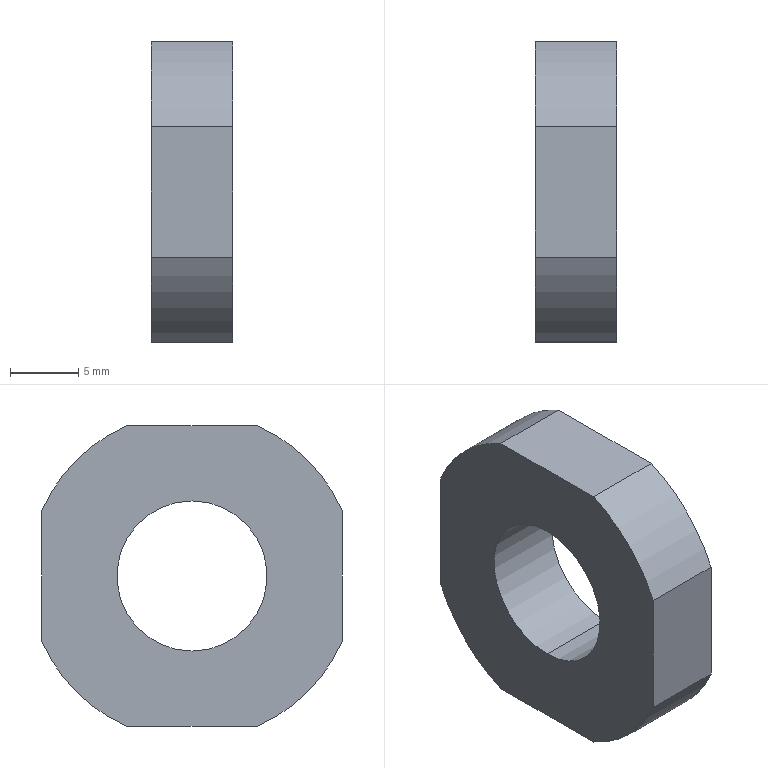Part | STEP file | PN_0031 locking nut | 1 solid | 12 faces | box 6 x 22 x 22 mm | volume 1989 mm3 | cylinder 6 | plane 6 | commonest cylinder face diameters 24 x4 11 x2
STEP:
#1=CARTESIAN_POINT('',(0.,0.,0.));
#2=DIRECTION('',(0.,0.,1.));
#3=DIRECTION('',(1.,0.,0.));
#4=AXIS2_PLACEMENT_3D('',#1,#2,#3);
#5=CARTESIAN_POINT('',(0.,0.,5.5));
#6=VERTEX_POINT('',#5);
#7=CARTESIAN_POINT('',(-6.,0.,5.5));
#8=VERTEX_POINT('',#7);
#9=CARTESIAN_POINT('',(0.,0.,5.5));
#10=DIRECTION('',(-1.,0.,0.));
#11=VECTOR('',#10,1.);
#12=LINE('',#9,#11);
#13=CARTESIAN_POINT('',(0.,0.,0.));
#14=DIRECTION('',(-1.,0.,0.));
#15=DIRECTION('',(0.,0.,1.));
#16=AXIS2_PLACEMENT_3D('',#13,#14,#15);
#17=CYLINDRICAL_SURFACE('',#16,5.5);
#18=CARTESIAN_POINT('',(6.283,0.));
#19=DIRECTION('',(0.,1.));
#20=VECTOR('',#19,1.);
#21=LINE('',#18,#20);
#22=(GEOMETRIC_REPRESENTATION_CONTEXT(2)PARAMETRIC_REPRESENTATION_CONTEXT()REPRESENTATION_CONTEXT('',''));
#23=DEFINITIONAL_REPRESENTATION('',(#21),#22);
#24=PCURVE('',#17,#23);
#25=CARTESIAN_POINT('',(0.,0.,0.));
#26=DIRECTION('',(-1.,0.,0.));
#27=DIRECTION('',(0.,0.,1.));
#28=AXIS2_PLACEMENT_3D('',#25,#26,#27);
#29=CYLINDRICAL_SURFACE('',#28,5.5);
#30=CARTESIAN_POINT('',(0.,0.));
#31=DIRECTION('',(0.,1.));
#32=VECTOR('',#31,1.);
#33=LINE('',#30,#32);
#34=(GEOMETRIC_REPRESENTATION_CONTEXT(2)PARAMETRIC_REPRESENTATION_CONTEXT()REPRESENTATION_CONTEXT('',''));
#35=DEFINITIONAL_REPRESENTATION('',(#33),#34);
#36=PCURVE('',#29,#35);
#37=SURFACE_CURVE('',#12,(#24,#36),.PCURVE_S1.);
#38=EDGE_CURVE('',#6,#8,#37,.T.);
#39=ORIENTED_EDGE('',*,*,#38,.T.);
#40=CARTESIAN_POINT('',(-6.,0.,-5.5));
#41=VERTEX_POINT('',#40);
#42=CARTESIAN_POINT('',(-6.,0.,0.));
#43=DIRECTION('',(1.,0.,0.));
#44=DIRECTION('',(0.,0.,-1.));
#45=AXIS2_PLACEMENT_3D('',#42,#43,#44);
#46=CIRCLE('',#45,5.5);
#47=CARTESIAN_POINT('',(9.425,6.));
#48=DIRECTION('',(-1.,0.));
#49=VECTOR('',#48,1.);
#50=LINE('',#47,#49);
#51=(GEOMETRIC_REPRESENTATION_CONTEXT(2)PARAMETRIC_REPRESENTATION_CONTEXT()REPRESENTATION_CONTEXT('',''));
#52=DEFINITIONAL_REPRESENTATION('',(#50),#51);
#53=PCURVE('',#17,#52);
#54=CARTESIAN_POINT('',(-6.,12.,0.));
#55=DIRECTION('',(-1.,0.,0.));
#56=DIRECTION('',(0.,0.,1.));
#57=AXIS2_PLACEMENT_3D('',#54,#55,#56);
#58=PLANE('',#57);
#59=CARTESIAN_POINT('',(-5.5,-12.));
#60=CARTESIAN_POINT('',(-5.5,-2.474));
#61=CARTESIAN_POINT('',(2.75,-7.237));
#62=CARTESIAN_POINT('',(11.,-12.));
#63=CARTESIAN_POINT('',(2.75,-16.763));
#64=CARTESIAN_POINT('',(-5.5,-21.526));
#65=CARTESIAN_POINT('',(-5.5,-12.));
#66=(BOUNDED_CURVE()B_SPLINE_CURVE(2,(#59,#60,#61,#62,#63,#64,#65),.UNSPECIFIED.,.T.,.F.)B_SPLINE_CURVE_WITH_KNOTS((1,2,2,2,2,1),(-2.094,0.,2.094,4.189,6.283,8.378),.UNSPECIFIED.)CURVE()GEOMETRIC_REPRESENTATION_ITEM()RATIONAL_B_SPLINE_CURVE((1.,0.5,1.,0.5,1.,0.5,1.))REPRESENTATION_ITEM(''));
#67=(GEOMETRIC_REPRESENTATION_CONTEXT(2)PARAMETRIC_REPRESENTATION_CONTEXT()REPRESENTATION_CONTEXT('',''));
#68=DEFINITIONAL_REPRESENTATION('',(#66),#67);
#69=PCURVE('',#58,#68);
#70=SURFACE_CURVE('',#46,(#53,#69),.PCURVE_S1.);
#71=EDGE_CURVE('',#8,#41,#70,.T.);
#72=ORIENTED_EDGE('',*,*,#71,.T.);
#73=CARTESIAN_POINT('',(0.,0.,-5.5));
#74=VERTEX_POINT('',#73);
#75=CARTESIAN_POINT('',(0.,0.,-5.5));
#76=DIRECTION('',(-1.,0.,0.));
#77=VECTOR('',#76,1.);
#78=LINE('',#75,#77);
#79=CARTESIAN_POINT('',(3.142,0.));
#80=DIRECTION('',(0.,1.));
#81=VECTOR('',#80,1.);
#82=LINE('',#79,#81);
#83=(GEOMETRIC_REPRESENTATION_CONTEXT(2)PARAMETRIC_REPRESENTATION_CONTEXT()REPRESENTATION_CONTEXT('',''));
#84=DEFINITIONAL_REPRESENTATION('',(#82),#83);
#85=PCURVE('',#17,#84);
#86=CARTESIAN_POINT('',(3.142,0.));
#87=DIRECTION('',(0.,1.));
#88=VECTOR('',#87,1.);
#89=LINE('',#86,#88);
#90=(GEOMETRIC_REPRESENTATION_CONTEXT(2)PARAMETRIC_REPRESENTATION_CONTEXT()REPRESENTATION_CONTEXT('',''));
#91=DEFINITIONAL_REPRESENTATION('',(#89),#90);
#92=PCURVE('',#29,#91);
#93=SURFACE_CURVE('',#78,(#85,#92),.PCURVE_S1.);
#94=EDGE_CURVE('',#74,#41,#93,.T.);
#95=ORIENTED_EDGE('',*,*,#94,.F.);
#96=CARTESIAN_POINT('',(0.,0.,0.));
#97=DIRECTION('',(1.,0.,0.));
#98=DIRECTION('',(0.,0.,-1.));
#99=AXIS2_PLACEMENT_3D('',#96,#97,#98);
#100=CIRCLE('',#99,5.5);
#101=CARTESIAN_POINT('',(9.425,0.));
#102=DIRECTION('',(-1.,0.));
#103=VECTOR('',#102,1.);
#104=LINE('',#101,#103);
#105=(GEOMETRIC_REPRESENTATION_CONTEXT(2)PARAMETRIC_REPRESENTATION_CONTEXT()REPRESENTATION_CONTEXT('',''));
#106=DEFINITIONAL_REPRESENTATION('',(#104),#105);
#107=PCURVE('',#17,#106);
#108=CARTESIAN_POINT('',(0.,0.,0.));
#109=DIRECTION('',(1.,0.,0.));
#110=DIRECTION('',(0.,0.,-1.));
#111=AXIS2_PLACEMENT_3D('',#108,#109,#110);
#112=PLANE('',#111);
#113=CARTESIAN_POINT('',(0.,0.));
#114=DIRECTION('',(1.,0.));
#115=AXIS2_PLACEMENT_2D('',#113,#114);
#116=CIRCLE('',#115,5.5);
#117=(GEOMETRIC_REPRESENTATION_CONTEXT(2)PARAMETRIC_REPRESENTATION_CONTEXT()REPRESENTATION_CONTEXT('',''));
#118=DEFINITIONAL_REPRESENTATION('',(#116),#117);
#119=PCURVE('',#112,#118);
#120=SURFACE_CURVE('',#100,(#107,#119),.PCURVE_S1.);
#121=EDGE_CURVE('',#6,#74,#120,.T.);
#122=ORIENTED_EDGE('',*,*,#121,.F.);
#123=EDGE_LOOP('',(#39,#72,#95,#122));
#124=FACE_BOUND('',#123,.F.);
#125=ADVANCED_FACE('',(#124),#17,.F.);
#126=CARTESIAN_POINT('',(0.,4.796,11.));
#127=VERTEX_POINT('',#126);
#128=CARTESIAN_POINT('',(-6.,4.796,11.));
#129=VERTEX_POINT('',#128);
#130=CARTESIAN_POINT('',(0.,4.796,11.));
#131=DIRECTION('',(-1.,0.,0.));
#132=VECTOR('',#131,1.);
#133=LINE('',#130,#132);
#134=CARTESIAN_POINT('',(0.,0.,0.));
#135=DIRECTION('',(1.,0.,0.));
#136=DIRECTION('',(0.,0.,-1.));
#137=AXIS2_PLACEMENT_3D('',#134,#135,#136);
#138=CYLINDRICAL_SURFACE('',#137,12.);
#139=CARTESIAN_POINT('',(2.73,0.));
#140=DIRECTION('',(0.,-1.));
#141=VECTOR('',#140,1.);
#142=LINE('',#139,#141);
#143=(GEOMETRIC_REPRESENTATION_CONTEXT(2)PARAMETRIC_REPRESENTATION_CONTEXT()REPRESENTATION_CONTEXT('',''));
#144=DEFINITIONAL_REPRESENTATION('',(#142),#143);
#145=PCURVE('',#138,#144);
#146=CARTESIAN_POINT('',(0.,17.205,11.));
#147=DIRECTION('',(0.,0.,-1.));
#148=DIRECTION('',(0.,1.,0.));
#149=AXIS2_PLACEMENT_3D('',#146,#147,#148);
#150=PLANE('',#149);
#151=CARTESIAN_POINT('',(-12.409,0.));
#152=DIRECTION('',(0.,-1.));
#153=VECTOR('',#152,1.);
#154=LINE('',#151,#153);
#155=(GEOMETRIC_REPRESENTATION_CONTEXT(2)PARAMETRIC_REPRESENTATION_CONTEXT()REPRESENTATION_CONTEXT('',''));
#156=DEFINITIONAL_REPRESENTATION('',(#154),#155);
#157=PCURVE('',#150,#156);
#158=SURFACE_CURVE('',#133,(#145,#157),.PCURVE_S1.);
#159=EDGE_CURVE('',#127,#129,#158,.T.);
#160=ORIENTED_EDGE('',*,*,#159,.F.);
#161=CARTESIAN_POINT('',(0.,11.,4.796));
#162=VERTEX_POINT('',#161);
#163=CARTESIAN_POINT('',(0.,0.,0.));
#164=DIRECTION('',(1.,0.,0.));
#165=DIRECTION('',(0.,0.,-1.));
#166=AXIS2_PLACEMENT_3D('',#163,#164,#165);
#167=CIRCLE('',#166,12.);
#168=CARTESIAN_POINT('',(0.,0.));
#169=DIRECTION('',(1.,0.));
#170=VECTOR('',#169,1.);
#171=LINE('',#168,#170);
#172=(GEOMETRIC_REPRESENTATION_CONTEXT(2)PARAMETRIC_REPRESENTATION_CONTEXT()REPRESENTATION_CONTEXT('',''));
#173=DEFINITIONAL_REPRESENTATION('',(#171),#172);
#174=PCURVE('',#138,#173);
#175=CARTESIAN_POINT('',(0.,0.));
#176=DIRECTION('',(1.,0.));
#177=AXIS2_PLACEMENT_2D('',#175,#176);
#178=CIRCLE('',#177,12.);
#179=(GEOMETRIC_REPRESENTATION_CONTEXT(2)PARAMETRIC_REPRESENTATION_CONTEXT()REPRESENTATION_CONTEXT('',''));
#180=DEFINITIONAL_REPRESENTATION('',(#178),#179);
#181=PCURVE('',#112,#180);
#182=SURFACE_CURVE('',#167,(#174,#181),.PCURVE_S1.);
#183=EDGE_CURVE('',#162,#127,#182,.T.);
#184=ORIENTED_EDGE('',*,*,#183,.F.);
#185=CARTESIAN_POINT('',(-6.,11.,4.796));
#186=VERTEX_POINT('',#185);
#187=CARTESIAN_POINT('',(0.,11.,4.796));
#188=DIRECTION('',(1.,0.,0.));
#189=VECTOR('',#188,1.);
#190=LINE('',#187,#189);
#191=CARTESIAN_POINT('',(1.982,0.));
#192=DIRECTION('',(0.,1.));
#193=VECTOR('',#192,1.);
#194=LINE('',#191,#193);
#195=(GEOMETRIC_REPRESENTATION_CONTEXT(2)PARAMETRIC_REPRESENTATION_CONTEXT()REPRESENTATION_CONTEXT('',''));
#196=DEFINITIONAL_REPRESENTATION('',(#194),#195);
#197=PCURVE('',#138,#196);
#198=CARTESIAN_POINT('',(0.,11.,-20.296));
#199=DIRECTION('',(0.,-1.,0.));
#200=DIRECTION('',(0.,0.,-1.));
#201=AXIS2_PLACEMENT_3D('',#198,#199,#200);
#202=PLANE('',#201);
#203=CARTESIAN_POINT('',(-25.092,0.));
#204=DIRECTION('',(0.,1.));
#205=VECTOR('',#204,1.);
#206=LINE('',#203,#205);
#207=(GEOMETRIC_REPRESENTATION_CONTEXT(2)PARAMETRIC_REPRESENTATION_CONTEXT()REPRESENTATION_CONTEXT('',''));
#208=DEFINITIONAL_REPRESENTATION('',(#206),#207);
#209=PCURVE('',#202,#208);
#210=SURFACE_CURVE('',#190,(#197,#209),.PCURVE_S1.);
#211=EDGE_CURVE('',#186,#162,#210,.T.);
#212=ORIENTED_EDGE('',*,*,#211,.F.);
#213=CARTESIAN_POINT('',(-6.,0.,0.));
#214=DIRECTION('',(1.,0.,0.));
#215=DIRECTION('',(0.,0.,-1.));
#216=AXIS2_PLACEMENT_3D('',#213,#214,#215);
#217=CIRCLE('',#216,12.);
#218=CARTESIAN_POINT('',(0.,-6.));
#219=DIRECTION('',(1.,0.));
#220=VECTOR('',#219,1.);
#221=LINE('',#218,#220);
#222=(GEOMETRIC_REPRESENTATION_CONTEXT(2)PARAMETRIC_REPRESENTATION_CONTEXT()REPRESENTATION_CONTEXT('',''));
#223=DEFINITIONAL_REPRESENTATION('',(#221),#222);
#224=PCURVE('',#138,#223);
#225=CARTESIAN_POINT('',(-12.,-12.));
#226=CARTESIAN_POINT('',(-12.,8.785));
#227=CARTESIAN_POINT('',(6.,-1.608));
#228=CARTESIAN_POINT('',(24.,-12.));
#229=CARTESIAN_POINT('',(6.,-22.392));
#230=CARTESIAN_POINT('',(-12.,-32.785));
#231=CARTESIAN_POINT('',(-12.,-12.));
#232=(BOUNDED_CURVE()B_SPLINE_CURVE(2,(#225,#226,#227,#228,#229,#230,#231),.UNSPECIFIED.,.T.,.F.)B_SPLINE_CURVE_WITH_KNOTS((1,2,2,2,2,1),(-2.094,0.,2.094,4.189,6.283,8.378),.UNSPECIFIED.)CURVE()GEOMETRIC_REPRESENTATION_ITEM()RATIONAL_B_SPLINE_CURVE((1.,0.5,1.,0.5,1.,0.5,1.))REPRESENTATION_ITEM(''));
#233=(GEOMETRIC_REPRESENTATION_CONTEXT(2)PARAMETRIC_REPRESENTATION_CONTEXT()REPRESENTATION_CONTEXT('',''));
#234=DEFINITIONAL_REPRESENTATION('',(#232),#233);
#235=PCURVE('',#58,#234);
#236=SURFACE_CURVE('',#217,(#224,#235),.PCURVE_S1.);
#237=EDGE_CURVE('',#186,#129,#236,.T.);
#238=ORIENTED_EDGE('',*,*,#237,.T.);
#239=EDGE_LOOP('',(#160,#184,#212,#238));
#240=FACE_BOUND('',#239,.T.);
#241=ADVANCED_FACE('',(#240),#138,.T.);
#242=CARTESIAN_POINT('',(0.,-4.796,-11.));
#243=VERTEX_POINT('',#242);
#244=CARTESIAN_POINT('',(-6.,-4.796,-11.));
#245=VERTEX_POINT('',#244);
#246=CARTESIAN_POINT('',(0.,-4.796,-11.));
#247=DIRECTION('',(-1.,0.,0.));
#248=VECTOR('',#247,1.);
#249=LINE('',#246,#248);
#250=CARTESIAN_POINT('',(0.,0.,0.));
#251=DIRECTION('',(1.,0.,0.));
#252=DIRECTION('',(0.,0.,-1.));
#253=AXIS2_PLACEMENT_3D('',#250,#251,#252);
#254=CYLINDRICAL_SURFACE('',#253,12.);
#255=CARTESIAN_POINT('',(5.872,0.));
#256=DIRECTION('',(0.,-1.));
#257=VECTOR('',#256,1.);
#258=LINE('',#255,#257);
#259=(GEOMETRIC_REPRESENTATION_CONTEXT(2)PARAMETRIC_REPRESENTATION_CONTEXT()REPRESENTATION_CONTEXT('',''));
#260=DEFINITIONAL_REPRESENTATION('',(#258),#259);
#261=PCURVE('',#254,#260);
#262=CARTESIAN_POINT('',(0.,17.205,-11.));
#263=DIRECTION('',(0.,0.,1.));
#264=DIRECTION('',(0.,-1.,0.));
#265=AXIS2_PLACEMENT_3D('',#262,#263,#264);
#266=PLANE('',#265);
#267=CARTESIAN_POINT('',(22.001,0.));
#268=DIRECTION('',(0.,-1.));
#269=VECTOR('',#268,1.);
#270=LINE('',#267,#269);
#271=(GEOMETRIC_REPRESENTATION_CONTEXT(2)PARAMETRIC_REPRESENTATION_CONTEXT()REPRESENTATION_CONTEXT('',''));
#272=DEFINITIONAL_REPRESENTATION('',(#270),#271);
#273=PCURVE('',#266,#272);
#274=SURFACE_CURVE('',#249,(#261,#273),.PCURVE_S1.);
#275=EDGE_CURVE('',#243,#245,#274,.T.);
#276=ORIENTED_EDGE('',*,*,#275,.F.);
#277=CARTESIAN_POINT('',(0.,-11.,-4.796));
#278=VERTEX_POINT('',#277);
#279=CARTESIAN_POINT('',(0.,0.,0.));
#280=DIRECTION('',(1.,0.,0.));
#281=DIRECTION('',(0.,0.,-1.));
#282=AXIS2_PLACEMENT_3D('',#279,#280,#281);
#283=CIRCLE('',#282,12.);
#284=CARTESIAN_POINT('',(0.,0.));
#285=DIRECTION('',(1.,0.));
#286=VECTOR('',#285,1.);
#287=LINE('',#284,#286);
#288=(GEOMETRIC_REPRESENTATION_CONTEXT(2)PARAMETRIC_REPRESENTATION_CONTEXT()REPRESENTATION_CONTEXT('',''));
#289=DEFINITIONAL_REPRESENTATION('',(#287),#288);
#290=PCURVE('',#254,#289);
#291=CARTESIAN_POINT('',(0.,0.));
#292=DIRECTION('',(1.,0.));
#293=AXIS2_PLACEMENT_2D('',#291,#292);
#294=CIRCLE('',#293,12.);
#295=(GEOMETRIC_REPRESENTATION_CONTEXT(2)PARAMETRIC_REPRESENTATION_CONTEXT()REPRESENTATION_CONTEXT('',''));
#296=DEFINITIONAL_REPRESENTATION('',(#294),#295);
#297=PCURVE('',#112,#296);
#298=SURFACE_CURVE('',#283,(#290,#297),.PCURVE_S1.);
#299=EDGE_CURVE('',#278,#243,#298,.T.);
#300=ORIENTED_EDGE('',*,*,#299,.F.);
#301=CARTESIAN_POINT('',(-6.,-11.,-4.796));
#302=VERTEX_POINT('',#301);
#303=CARTESIAN_POINT('',(0.,-11.,-4.796));
#304=DIRECTION('',(1.,0.,0.));
#305=VECTOR('',#304,1.);
#306=LINE('',#303,#305);
#307=CARTESIAN_POINT('',(5.124,0.));
#308=DIRECTION('',(0.,1.));
#309=VECTOR('',#308,1.);
#310=LINE('',#307,#309);
#311=(GEOMETRIC_REPRESENTATION_CONTEXT(2)PARAMETRIC_REPRESENTATION_CONTEXT()REPRESENTATION_CONTEXT('',''));
#312=DEFINITIONAL_REPRESENTATION('',(#310),#311);
#313=PCURVE('',#254,#312);
#314=CARTESIAN_POINT('',(0.,-11.,-20.296));
#315=DIRECTION('',(0.,1.,0.));
#316=DIRECTION('',(0.,0.,1.));
#317=AXIS2_PLACEMENT_3D('',#314,#315,#316);
#318=PLANE('',#317);
#319=CARTESIAN_POINT('',(15.501,0.));
#320=DIRECTION('',(0.,1.));
#321=VECTOR('',#320,1.);
#322=LINE('',#319,#321);
#323=(GEOMETRIC_REPRESENTATION_CONTEXT(2)PARAMETRIC_REPRESENTATION_CONTEXT()REPRESENTATION_CONTEXT('',''));
#324=DEFINITIONAL_REPRESENTATION('',(#322),#323);
#325=PCURVE('',#318,#324);
#326=SURFACE_CURVE('',#306,(#313,#325),.PCURVE_S1.);
#327=EDGE_CURVE('',#302,#278,#326,.T.);
#328=ORIENTED_EDGE('',*,*,#327,.F.);
#329=CARTESIAN_POINT('',(-6.,0.,0.));
#330=DIRECTION('',(1.,0.,0.));
#331=DIRECTION('',(0.,0.,-1.));
#332=AXIS2_PLACEMENT_3D('',#329,#330,#331);
#333=CIRCLE('',#332,12.);
#334=CARTESIAN_POINT('',(0.,-6.));
#335=DIRECTION('',(1.,0.));
#336=VECTOR('',#335,1.);
#337=LINE('',#334,#336);
#338=(GEOMETRIC_REPRESENTATION_CONTEXT(2)PARAMETRIC_REPRESENTATION_CONTEXT()REPRESENTATION_CONTEXT('',''));
#339=DEFINITIONAL_REPRESENTATION('',(#337),#338);
#340=PCURVE('',#254,#339);
#341=CARTESIAN_POINT('',(-12.,-12.));
#342=CARTESIAN_POINT('',(-12.,8.785));
#343=CARTESIAN_POINT('',(6.,-1.608));
#344=CARTESIAN_POINT('',(24.,-12.));
#345=CARTESIAN_POINT('',(6.,-22.392));
#346=CARTESIAN_POINT('',(-12.,-32.785));
#347=CARTESIAN_POINT('',(-12.,-12.));
#348=(BOUNDED_CURVE()B_SPLINE_CURVE(2,(#341,#342,#343,#344,#345,#346,#347),.UNSPECIFIED.,.T.,.F.)B_SPLINE_CURVE_WITH_KNOTS((1,2,2,2,2,1),(-2.094,0.,2.094,4.189,6.283,8.378),.UNSPECIFIED.)CURVE()GEOMETRIC_REPRESENTATION_ITEM()RATIONAL_B_SPLINE_CURVE((1.,0.5,1.,0.5,1.,0.5,1.))REPRESENTATION_ITEM(''));
#349=(GEOMETRIC_REPRESENTATION_CONTEXT(2)PARAMETRIC_REPRESENTATION_CONTEXT()REPRESENTATION_CONTEXT('',''));
#350=DEFINITIONAL_REPRESENTATION('',(#348),#349);
#351=PCURVE('',#58,#350);
#352=SURFACE_CURVE('',#333,(#340,#351),.PCURVE_S1.);
#353=EDGE_CURVE('',#302,#245,#352,.T.);
#354=ORIENTED_EDGE('',*,*,#353,.T.);
#355=EDGE_LOOP('',(#276,#300,#328,#354));
#356=FACE_BOUND('',#355,.T.);
#357=ADVANCED_FACE('',(#356),#254,.T.);
#358=CARTESIAN_POINT('',(-6.,-4.796,11.));
#359=VERTEX_POINT('',#358);
#360=CARTESIAN_POINT('',(0.,-4.796,11.));
#361=VERTEX_POINT('',#360);
#362=CARTESIAN_POINT('',(0.,-4.796,11.));
#363=DIRECTION('',(1.,0.,0.));
#364=VECTOR('',#363,1.);
#365=LINE('',#362,#364);
#366=CARTESIAN_POINT('',(0.,0.,0.));
#367=DIRECTION('',(1.,0.,0.));
#368=DIRECTION('',(0.,0.,-1.));
#369=AXIS2_PLACEMENT_3D('',#366,#367,#368);
#370=CYLINDRICAL_SURFACE('',#369,12.);
#371=CARTESIAN_POINT('',(3.553,0.));
#372=DIRECTION('',(0.,1.));
#373=VECTOR('',#372,1.);
#374=LINE('',#371,#373);
#375=(GEOMETRIC_REPRESENTATION_CONTEXT(2)PARAMETRIC_REPRESENTATION_CONTEXT()REPRESENTATION_CONTEXT('',''));
#376=DEFINITIONAL_REPRESENTATION('',(#374),#375);
#377=PCURVE('',#370,#376);
#378=CARTESIAN_POINT('',(-22.001,0.));
#379=DIRECTION('',(0.,1.));
#380=VECTOR('',#379,1.);
#381=LINE('',#378,#380);
#382=(GEOMETRIC_REPRESENTATION_CONTEXT(2)PARAMETRIC_REPRESENTATION_CONTEXT()REPRESENTATION_CONTEXT('',''));
#383=DEFINITIONAL_REPRESENTATION('',(#381),#382);
#384=PCURVE('',#150,#383);
#385=SURFACE_CURVE('',#365,(#377,#384),.PCURVE_S1.);
#386=EDGE_CURVE('',#359,#361,#385,.T.);
#387=ORIENTED_EDGE('',*,*,#386,.F.);
#388=CARTESIAN_POINT('',(-6.,-11.,4.796));
#389=VERTEX_POINT('',#388);
#390=CARTESIAN_POINT('',(-6.,0.,0.));
#391=DIRECTION('',(1.,0.,0.));
#392=DIRECTION('',(0.,0.,-1.));
#393=AXIS2_PLACEMENT_3D('',#390,#391,#392);
#394=CIRCLE('',#393,12.);
#395=CARTESIAN_POINT('',(0.,-6.));
#396=DIRECTION('',(1.,0.));
#397=VECTOR('',#396,1.);
#398=LINE('',#395,#397);
#399=(GEOMETRIC_REPRESENTATION_CONTEXT(2)PARAMETRIC_REPRESENTATION_CONTEXT()REPRESENTATION_CONTEXT('',''));
#400=DEFINITIONAL_REPRESENTATION('',(#398),#399);
#401=PCURVE('',#370,#400);
#402=CARTESIAN_POINT('',(-12.,-12.));
#403=CARTESIAN_POINT('',(-12.,8.785));
#404=CARTESIAN_POINT('',(6.,-1.608));
#405=CARTESIAN_POINT('',(24.,-12.));
#406=CARTESIAN_POINT('',(6.,-22.392));
#407=CARTESIAN_POINT('',(-12.,-32.785));
#408=CARTESIAN_POINT('',(-12.,-12.));
#409=(BOUNDED_CURVE()B_SPLINE_CURVE(2,(#402,#403,#404,#405,#406,#407,#408),.UNSPECIFIED.,.T.,.F.)B_SPLINE_CURVE_WITH_KNOTS((1,2,2,2,2,1),(-2.094,0.,2.094,4.189,6.283,8.378),.UNSPECIFIED.)CURVE()GEOMETRIC_REPRESENTATION_ITEM()RATIONAL_B_SPLINE_CURVE((1.,0.5,1.,0.5,1.,0.5,1.))REPRESENTATION_ITEM(''));
#410=(GEOMETRIC_REPRESENTATION_CONTEXT(2)PARAMETRIC_REPRESENTATION_CONTEXT()REPRESENTATION_CONTEXT('',''));
#411=DEFINITIONAL_REPRESENTATION('',(#409),#410);
#412=PCURVE('',#58,#411);
#413=SURFACE_CURVE('',#394,(#401,#412),.PCURVE_S1.);
#414=EDGE_CURVE('',#359,#389,#413,.T.);
#415=ORIENTED_EDGE('',*,*,#414,.T.);
#416=CARTESIAN_POINT('',(0.,-11.,4.796));
#417=VERTEX_POINT('',#416);
#418=CARTESIAN_POINT('',(0.,-11.,4.796));
#419=DIRECTION('',(-1.,0.,0.));
#420=VECTOR('',#419,1.);
#421=LINE('',#418,#420);
#422=CARTESIAN_POINT('',(4.301,0.));
#423=DIRECTION('',(0.,-1.));
#424=VECTOR('',#423,1.);
#425=LINE('',#422,#424);
#426=(GEOMETRIC_REPRESENTATION_CONTEXT(2)PARAMETRIC_REPRESENTATION_CONTEXT()REPRESENTATION_CONTEXT('',''));
#427=DEFINITIONAL_REPRESENTATION('',(#425),#426);
#428=PCURVE('',#370,#427);
#429=CARTESIAN_POINT('',(25.092,0.));
#430=DIRECTION('',(0.,-1.));
#431=VECTOR('',#430,1.);
#432=LINE('',#429,#431);
#433=(GEOMETRIC_REPRESENTATION_CONTEXT(2)PARAMETRIC_REPRESENTATION_CONTEXT()REPRESENTATION_CONTEXT('',''));
#434=DEFINITIONAL_REPRESENTATION('',(#432),#433);
#435=PCURVE('',#318,#434);
#436=SURFACE_CURVE('',#421,(#428,#435),.PCURVE_S1.);
#437=EDGE_CURVE('',#417,#389,#436,.T.);
#438=ORIENTED_EDGE('',*,*,#437,.F.);
#439=CARTESIAN_POINT('',(0.,0.,0.));
#440=DIRECTION('',(1.,0.,0.));
#441=DIRECTION('',(0.,0.,-1.));
#442=AXIS2_PLACEMENT_3D('',#439,#440,#441);
#443=CIRCLE('',#442,12.);
#444=CARTESIAN_POINT('',(0.,0.));
#445=DIRECTION('',(1.,0.));
#446=VECTOR('',#445,1.);
#447=LINE('',#444,#446);
#448=(GEOMETRIC_REPRESENTATION_CONTEXT(2)PARAMETRIC_REPRESENTATION_CONTEXT()REPRESENTATION_CONTEXT('',''));
#449=DEFINITIONAL_REPRESENTATION('',(#447),#448);
#450=PCURVE('',#370,#449);
#451=CARTESIAN_POINT('',(0.,0.));
#452=DIRECTION('',(1.,0.));
#453=AXIS2_PLACEMENT_2D('',#451,#452);
#454=CIRCLE('',#453,12.);
#455=(GEOMETRIC_REPRESENTATION_CONTEXT(2)PARAMETRIC_REPRESENTATION_CONTEXT()REPRESENTATION_CONTEXT('',''));
#456=DEFINITIONAL_REPRESENTATION('',(#454),#455);
#457=PCURVE('',#112,#456);
#458=SURFACE_CURVE('',#443,(#450,#457),.PCURVE_S1.);
#459=EDGE_CURVE('',#361,#417,#458,.T.);
#460=ORIENTED_EDGE('',*,*,#459,.F.);
#461=EDGE_LOOP('',(#387,#415,#438,#460));
#462=FACE_BOUND('',#461,.T.);
#463=ADVANCED_FACE('',(#462),#370,.T.);
#464=CARTESIAN_POINT('',(0.,17.205,11.));
#465=DIRECTION('',(0.,-1.,0.));
#466=VECTOR('',#465,1.);
#467=LINE('',#464,#466);
#468=CARTESIAN_POINT('',(-11.,17.205));
#469=DIRECTION('',(0.,-1.));
#470=VECTOR('',#469,1.);
#471=LINE('',#468,#470);
#472=(GEOMETRIC_REPRESENTATION_CONTEXT(2)PARAMETRIC_REPRESENTATION_CONTEXT()REPRESENTATION_CONTEXT('',''));
#473=DEFINITIONAL_REPRESENTATION('',(#471),#472);
#474=PCURVE('',#112,#473);
#475=CARTESIAN_POINT('',(0.,0.));
#476=DIRECTION('',(-1.,0.));
#477=VECTOR('',#476,1.);
#478=LINE('',#475,#477);
#479=(GEOMETRIC_REPRESENTATION_CONTEXT(2)PARAMETRIC_REPRESENTATION_CONTEXT()REPRESENTATION_CONTEXT('',''));
#480=DEFINITIONAL_REPRESENTATION('',(#478),#479);
#481=PCURVE('',#150,#480);
#482=SURFACE_CURVE('',#467,(#474,#481),.PCURVE_S1.);
#483=EDGE_CURVE('',#127,#361,#482,.T.);
#484=ORIENTED_EDGE('',*,*,#483,.T.);
#485=ORIENTED_EDGE('',*,*,#459,.T.);
#486=CARTESIAN_POINT('',(0.,-11.,-20.296));
#487=DIRECTION('',(0.,0.,-1.));
#488=VECTOR('',#487,1.);
#489=LINE('',#486,#488);
#490=CARTESIAN_POINT('',(20.296,-11.));
#491=DIRECTION('',(1.,0.));
#492=VECTOR('',#491,1.);
#493=LINE('',#490,#492);
#494=(GEOMETRIC_REPRESENTATION_CONTEXT(2)PARAMETRIC_REPRESENTATION_CONTEXT()REPRESENTATION_CONTEXT('',''));
#495=DEFINITIONAL_REPRESENTATION('',(#493),#494);
#496=PCURVE('',#112,#495);
#497=CARTESIAN_POINT('',(0.,0.));
#498=DIRECTION('',(-1.,0.));
#499=VECTOR('',#498,1.);
#500=LINE('',#497,#499);
#501=(GEOMETRIC_REPRESENTATION_CONTEXT(2)PARAMETRIC_REPRESENTATION_CONTEXT()REPRESENTATION_CONTEXT('',''));
#502=DEFINITIONAL_REPRESENTATION('',(#500),#501);
#503=PCURVE('',#318,#502);
#504=SURFACE_CURVE('',#489,(#496,#503),.PCURVE_S1.);
#505=EDGE_CURVE('',#417,#278,#504,.T.);
#506=ORIENTED_EDGE('',*,*,#505,.T.);
#507=ORIENTED_EDGE('',*,*,#299,.T.);
#508=CARTESIAN_POINT('',(0.,4.796,-11.));
#509=VERTEX_POINT('',#508);
#510=CARTESIAN_POINT('',(0.,17.205,-11.));
#511=DIRECTION('',(0.,1.,0.));
#512=VECTOR('',#511,1.);
#513=LINE('',#510,#512);
#514=CARTESIAN_POINT('',(11.,17.205));
#515=DIRECTION('',(0.,1.));
#516=VECTOR('',#515,1.);
#517=LINE('',#514,#516);
#518=(GEOMETRIC_REPRESENTATION_CONTEXT(2)PARAMETRIC_REPRESENTATION_CONTEXT()REPRESENTATION_CONTEXT('',''));
#519=DEFINITIONAL_REPRESENTATION('',(#517),#518);
#520=PCURVE('',#112,#519);
#521=CARTESIAN_POINT('',(0.,0.));
#522=DIRECTION('',(-1.,0.));
#523=VECTOR('',#522,1.);
#524=LINE('',#521,#523);
#525=(GEOMETRIC_REPRESENTATION_CONTEXT(2)PARAMETRIC_REPRESENTATION_CONTEXT()REPRESENTATION_CONTEXT('',''));
#526=DEFINITIONAL_REPRESENTATION('',(#524),#525);
#527=PCURVE('',#266,#526);
#528=SURFACE_CURVE('',#513,(#520,#527),.PCURVE_S1.);
#529=EDGE_CURVE('',#243,#509,#528,.T.);
#530=ORIENTED_EDGE('',*,*,#529,.T.);
#531=CARTESIAN_POINT('',(0.,11.,-4.796));
#532=VERTEX_POINT('',#531);
#533=CARTESIAN_POINT('',(0.,0.,0.));
#534=DIRECTION('',(1.,0.,0.));
#535=DIRECTION('',(0.,0.,-1.));
#536=AXIS2_PLACEMENT_3D('',#533,#534,#535);
#537=CIRCLE('',#536,12.);
#538=CARTESIAN_POINT('',(0.,0.));
#539=DIRECTION('',(1.,0.));
#540=AXIS2_PLACEMENT_2D('',#538,#539);
#541=CIRCLE('',#540,12.);
#542=(GEOMETRIC_REPRESENTATION_CONTEXT(2)PARAMETRIC_REPRESENTATION_CONTEXT()REPRESENTATION_CONTEXT('',''));
#543=DEFINITIONAL_REPRESENTATION('',(#541),#542);
#544=PCURVE('',#112,#543);
#545=CARTESIAN_POINT('',(0.,0.,0.));
#546=DIRECTION('',(1.,0.,0.));
#547=DIRECTION('',(0.,0.,-1.));
#548=AXIS2_PLACEMENT_3D('',#545,#546,#547);
#549=CYLINDRICAL_SURFACE('',#548,12.);
#550=CARTESIAN_POINT('',(0.,0.));
#551=DIRECTION('',(1.,0.));
#552=VECTOR('',#551,1.);
#553=LINE('',#550,#552);
#554=(GEOMETRIC_REPRESENTATION_CONTEXT(2)PARAMETRIC_REPRESENTATION_CONTEXT()REPRESENTATION_CONTEXT('',''));
#555=DEFINITIONAL_REPRESENTATION('',(#553),#554);
#556=PCURVE('',#549,#555);
#557=SURFACE_CURVE('',#537,(#544,#556),.PCURVE_S1.);
#558=EDGE_CURVE('',#509,#532,#557,.T.);
#559=ORIENTED_EDGE('',*,*,#558,.T.);
#560=CARTESIAN_POINT('',(0.,11.,-20.296));
#561=DIRECTION('',(0.,0.,1.));
#562=VECTOR('',#561,1.);
#563=LINE('',#560,#562);
#564=CARTESIAN_POINT('',(20.296,11.));
#565=DIRECTION('',(-1.,0.));
#566=VECTOR('',#565,1.);
#567=LINE('',#564,#566);
#568=(GEOMETRIC_REPRESENTATION_CONTEXT(2)PARAMETRIC_REPRESENTATION_CONTEXT()REPRESENTATION_CONTEXT('',''));
#569=DEFINITIONAL_REPRESENTATION('',(#567),#568);
#570=PCURVE('',#112,#569);
#571=CARTESIAN_POINT('',(0.,0.));
#572=DIRECTION('',(-1.,0.));
#573=VECTOR('',#572,1.);
#574=LINE('',#571,#573);
#575=(GEOMETRIC_REPRESENTATION_CONTEXT(2)PARAMETRIC_REPRESENTATION_CONTEXT()REPRESENTATION_CONTEXT('',''));
#576=DEFINITIONAL_REPRESENTATION('',(#574),#575);
#577=PCURVE('',#202,#576);
#578=SURFACE_CURVE('',#563,(#570,#577),.PCURVE_S1.);
#579=EDGE_CURVE('',#532,#162,#578,.T.);
#580=ORIENTED_EDGE('',*,*,#579,.T.);
#581=ORIENTED_EDGE('',*,*,#183,.T.);
#582=EDGE_LOOP('',(#484,#485,#506,#507,#530,#559,#580,#581));
#583=FACE_BOUND('',#582,.T.);
#584=ORIENTED_EDGE('',*,*,#121,.F.);
#585=CARTESIAN_POINT('',(0.,0.,0.));
#586=DIRECTION('',(1.,0.,0.));
#587=DIRECTION('',(0.,0.,-1.));
#588=AXIS2_PLACEMENT_3D('',#585,#586,#587);
#589=CIRCLE('',#588,5.5);
#590=CARTESIAN_POINT('',(0.,0.));
#591=DIRECTION('',(1.,0.));
#592=AXIS2_PLACEMENT_2D('',#590,#591);
#593=CIRCLE('',#592,5.5);
#594=(GEOMETRIC_REPRESENTATION_CONTEXT(2)PARAMETRIC_REPRESENTATION_CONTEXT()REPRESENTATION_CONTEXT('',''));
#595=DEFINITIONAL_REPRESENTATION('',(#593),#594);
#596=PCURVE('',#112,#595);
#597=CARTESIAN_POINT('',(3.142,0.));
#598=DIRECTION('',(-1.,0.));
#599=VECTOR('',#598,1.);
#600=LINE('',#597,#599);
#601=(GEOMETRIC_REPRESENTATION_CONTEXT(2)PARAMETRIC_REPRESENTATION_CONTEXT()REPRESENTATION_CONTEXT('',''));
#602=DEFINITIONAL_REPRESENTATION('',(#600),#601);
#603=PCURVE('',#29,#602);
#604=SURFACE_CURVE('',#589,(#596,#603),.PCURVE_S1.);
#605=EDGE_CURVE('',#74,#6,#604,.T.);
#606=ORIENTED_EDGE('',*,*,#605,.F.);
#607=EDGE_LOOP('',(#584,#606));
#608=FACE_BOUND('',#607,.T.);
#609=ADVANCED_FACE('',(#583,#608),#112,.T.);
#610=CARTESIAN_POINT('',(-6.,12.,11.));
#611=DIRECTION('',(0.,-1.,0.));
#612=VECTOR('',#611,1.);
#613=LINE('',#610,#612);
#614=CARTESIAN_POINT('',(11.,0.));
#615=DIRECTION('',(0.,-1.));
#616=VECTOR('',#615,1.);
#617=LINE('',#614,#616);
#618=(GEOMETRIC_REPRESENTATION_CONTEXT(2)PARAMETRIC_REPRESENTATION_CONTEXT()REPRESENTATION_CONTEXT('',''));
#619=DEFINITIONAL_REPRESENTATION('',(#617),#618);
#620=PCURVE('',#58,#619);
#621=CARTESIAN_POINT('',(-5.205,-6.));
#622=DIRECTION('',(-1.,0.));
#623=VECTOR('',#622,1.);
#624=LINE('',#621,#623);
#625=(GEOMETRIC_REPRESENTATION_CONTEXT(2)PARAMETRIC_REPRESENTATION_CONTEXT()REPRESENTATION_CONTEXT('',''));
#626=DEFINITIONAL_REPRESENTATION('',(#624),#625);
#627=PCURVE('',#150,#626);
#628=SURFACE_CURVE('',#613,(#620,#627),.PCURVE_S1.);
#629=EDGE_CURVE('',#129,#359,#628,.T.);
#630=ORIENTED_EDGE('',*,*,#629,.F.);
#631=ORIENTED_EDGE('',*,*,#237,.F.);
#632=CARTESIAN_POINT('',(-6.,11.,-4.796));
#633=VERTEX_POINT('',#632);
#634=CARTESIAN_POINT('',(-6.,11.,-20.296));
#635=DIRECTION('',(0.,0.,1.));
#636=VECTOR('',#635,1.);
#637=LINE('',#634,#636);
#638=CARTESIAN_POINT('',(-20.296,-1.));
#639=DIRECTION('',(1.,0.));
#640=VECTOR('',#639,1.);
#641=LINE('',#638,#640);
#642=(GEOMETRIC_REPRESENTATION_CONTEXT(2)PARAMETRIC_REPRESENTATION_CONTEXT()REPRESENTATION_CONTEXT('',''));
#643=DEFINITIONAL_REPRESENTATION('',(#641),#642);
#644=PCURVE('',#58,#643);
#645=CARTESIAN_POINT('',(0.,-6.));
#646=DIRECTION('',(-1.,0.));
#647=VECTOR('',#646,1.);
#648=LINE('',#645,#647);
#649=(GEOMETRIC_REPRESENTATION_CONTEXT(2)PARAMETRIC_REPRESENTATION_CONTEXT()REPRESENTATION_CONTEXT('',''));
#650=DEFINITIONAL_REPRESENTATION('',(#648),#649);
#651=PCURVE('',#202,#650);
#652=SURFACE_CURVE('',#637,(#644,#651),.PCURVE_S1.);
#653=EDGE_CURVE('',#633,#186,#652,.T.);
#654=ORIENTED_EDGE('',*,*,#653,.F.);
#655=CARTESIAN_POINT('',(-6.,4.796,-11.));
#656=VERTEX_POINT('',#655);
#657=CARTESIAN_POINT('',(-6.,0.,0.));
#658=DIRECTION('',(1.,0.,0.));
#659=DIRECTION('',(0.,0.,-1.));
#660=AXIS2_PLACEMENT_3D('',#657,#658,#659);
#661=CIRCLE('',#660,12.);
#662=CARTESIAN_POINT('',(-12.,-12.));
#663=CARTESIAN_POINT('',(-12.,8.785));
#664=CARTESIAN_POINT('',(6.,-1.608));
#665=CARTESIAN_POINT('',(24.,-12.));
#666=CARTESIAN_POINT('',(6.,-22.392));
#667=CARTESIAN_POINT('',(-12.,-32.785));
#668=CARTESIAN_POINT('',(-12.,-12.));
#669=(BOUNDED_CURVE()B_SPLINE_CURVE(2,(#662,#663,#664,#665,#666,#667,#668),.UNSPECIFIED.,.T.,.F.)B_SPLINE_CURVE_WITH_KNOTS((1,2,2,2,2,1),(-2.094,0.,2.094,4.189,6.283,8.378),.UNSPECIFIED.)CURVE()GEOMETRIC_REPRESENTATION_ITEM()RATIONAL_B_SPLINE_CURVE((1.,0.5,1.,0.5,1.,0.5,1.))REPRESENTATION_ITEM(''));
#670=(GEOMETRIC_REPRESENTATION_CONTEXT(2)PARAMETRIC_REPRESENTATION_CONTEXT()REPRESENTATION_CONTEXT('',''));
#671=DEFINITIONAL_REPRESENTATION('',(#669),#670);
#672=PCURVE('',#58,#671);
#673=CARTESIAN_POINT('',(0.,-6.));
#674=DIRECTION('',(1.,0.));
#675=VECTOR('',#674,1.);
#676=LINE('',#673,#675);
#677=(GEOMETRIC_REPRESENTATION_CONTEXT(2)PARAMETRIC_REPRESENTATION_CONTEXT()REPRESENTATION_CONTEXT('',''));
#678=DEFINITIONAL_REPRESENTATION('',(#676),#677);
#679=PCURVE('',#549,#678);
#680=SURFACE_CURVE('',#661,(#672,#679),.PCURVE_S1.);
#681=EDGE_CURVE('',#656,#633,#680,.T.);
#682=ORIENTED_EDGE('',*,*,#681,.F.);
#683=CARTESIAN_POINT('',(-6.,17.205,-11.));
#684=DIRECTION('',(0.,1.,0.));
#685=VECTOR('',#684,1.);
#686=LINE('',#683,#685);
#687=CARTESIAN_POINT('',(-11.,5.205));
#688=DIRECTION('',(0.,1.));
#689=VECTOR('',#688,1.);
#690=LINE('',#687,#689);
#691=(GEOMETRIC_REPRESENTATION_CONTEXT(2)PARAMETRIC_REPRESENTATION_CONTEXT()REPRESENTATION_CONTEXT('',''));
#692=DEFINITIONAL_REPRESENTATION('',(#690),#691);
#693=PCURVE('',#58,#692);
#694=CARTESIAN_POINT('',(0.,-6.));
#695=DIRECTION('',(-1.,0.));
#696=VECTOR('',#695,1.);
#697=LINE('',#694,#696);
#698=(GEOMETRIC_REPRESENTATION_CONTEXT(2)PARAMETRIC_REPRESENTATION_CONTEXT()REPRESENTATION_CONTEXT('',''));
#699=DEFINITIONAL_REPRESENTATION('',(#697),#698);
#700=PCURVE('',#266,#699);
#701=SURFACE_CURVE('',#686,(#693,#700),.PCURVE_S1.);
#702=EDGE_CURVE('',#245,#656,#701,.T.);
#703=ORIENTED_EDGE('',*,*,#702,.F.);
#704=ORIENTED_EDGE('',*,*,#353,.F.);
#705=CARTESIAN_POINT('',(-6.,-11.,-20.296));
#706=DIRECTION('',(0.,0.,-1.));
#707=VECTOR('',#706,1.);
#708=LINE('',#705,#707);
#709=CARTESIAN_POINT('',(-20.296,-23.));
#710=DIRECTION('',(-1.,0.));
#711=VECTOR('',#710,1.);
#712=LINE('',#709,#711);
#713=(GEOMETRIC_REPRESENTATION_CONTEXT(2)PARAMETRIC_REPRESENTATION_CONTEXT()REPRESENTATION_CONTEXT('',''));
#714=DEFINITIONAL_REPRESENTATION('',(#712),#713);
#715=PCURVE('',#58,#714);
#716=CARTESIAN_POINT('',(0.,-6.));
#717=DIRECTION('',(-1.,0.));
#718=VECTOR('',#717,1.);
#719=LINE('',#716,#718);
#720=(GEOMETRIC_REPRESENTATION_CONTEXT(2)PARAMETRIC_REPRESENTATION_CONTEXT()REPRESENTATION_CONTEXT('',''));
#721=DEFINITIONAL_REPRESENTATION('',(#719),#720);
#722=PCURVE('',#318,#721);
#723=SURFACE_CURVE('',#708,(#715,#722),.PCURVE_S1.);
#724=EDGE_CURVE('',#389,#302,#723,.T.);
#725=ORIENTED_EDGE('',*,*,#724,.F.);
#726=ORIENTED_EDGE('',*,*,#414,.F.);
#727=EDGE_LOOP('',(#630,#631,#654,#682,#703,#704,#725,#726));
#728=FACE_BOUND('',#727,.T.);
#729=ORIENTED_EDGE('',*,*,#71,.T.);
#730=CARTESIAN_POINT('',(-6.,0.,0.));
#731=DIRECTION('',(1.,0.,0.));
#732=DIRECTION('',(0.,0.,-1.));
#733=AXIS2_PLACEMENT_3D('',#730,#731,#732);
#734=CIRCLE('',#733,5.5);
#735=CARTESIAN_POINT('',(-5.5,-12.));
#736=CARTESIAN_POINT('',(-5.5,-2.474));
#737=CARTESIAN_POINT('',(2.75,-7.237));
#738=CARTESIAN_POINT('',(11.,-12.));
#739=CARTESIAN_POINT('',(2.75,-16.763));
#740=CARTESIAN_POINT('',(-5.5,-21.526));
#741=CARTESIAN_POINT('',(-5.5,-12.));
#742=(BOUNDED_CURVE()B_SPLINE_CURVE(2,(#735,#736,#737,#738,#739,#740,#741),.UNSPECIFIED.,.T.,.F.)B_SPLINE_CURVE_WITH_KNOTS((1,2,2,2,2,1),(-2.094,0.,2.094,4.189,6.283,8.378),.UNSPECIFIED.)CURVE()GEOMETRIC_REPRESENTATION_ITEM()RATIONAL_B_SPLINE_CURVE((1.,0.5,1.,0.5,1.,0.5,1.))REPRESENTATION_ITEM(''));
#743=(GEOMETRIC_REPRESENTATION_CONTEXT(2)PARAMETRIC_REPRESENTATION_CONTEXT()REPRESENTATION_CONTEXT('',''));
#744=DEFINITIONAL_REPRESENTATION('',(#742),#743);
#745=PCURVE('',#58,#744);
#746=CARTESIAN_POINT('',(3.142,6.));
#747=DIRECTION('',(-1.,0.));
#748=VECTOR('',#747,1.);
#749=LINE('',#746,#748);
#750=(GEOMETRIC_REPRESENTATION_CONTEXT(2)PARAMETRIC_REPRESENTATION_CONTEXT()REPRESENTATION_CONTEXT('',''));
#751=DEFINITIONAL_REPRESENTATION('',(#749),#750);
#752=PCURVE('',#29,#751);
#753=SURFACE_CURVE('',#734,(#745,#752),.PCURVE_S1.);
#754=EDGE_CURVE('',#41,#8,#753,.T.);
#755=ORIENTED_EDGE('',*,*,#754,.T.);
#756=EDGE_LOOP('',(#729,#755));
#757=FACE_BOUND('',#756,.T.);
#758=ADVANCED_FACE('',(#728,#757),#58,.T.);
#759=CARTESIAN_POINT('',(0.,4.796,-11.));
#760=DIRECTION('',(1.,0.,0.));
#761=VECTOR('',#760,1.);
#762=LINE('',#759,#761);
#763=CARTESIAN_POINT('',(0.4111,0.));
#764=DIRECTION('',(0.,1.));
#765=VECTOR('',#764,1.);
#766=LINE('',#763,#765);
#767=(GEOMETRIC_REPRESENTATION_CONTEXT(2)PARAMETRIC_REPRESENTATION_CONTEXT()REPRESENTATION_CONTEXT('',''));
#768=DEFINITIONAL_REPRESENTATION('',(#766),#767);
#769=PCURVE('',#549,#768);
#770=CARTESIAN_POINT('',(12.409,0.));
#771=DIRECTION('',(0.,1.));
#772=VECTOR('',#771,1.);
#773=LINE('',#770,#772);
#774=(GEOMETRIC_REPRESENTATION_CONTEXT(2)PARAMETRIC_REPRESENTATION_CONTEXT()REPRESENTATION_CONTEXT('',''));
#775=DEFINITIONAL_REPRESENTATION('',(#773),#774);
#776=PCURVE('',#266,#775);
#777=SURFACE_CURVE('',#762,(#769,#776),.PCURVE_S1.);
#778=EDGE_CURVE('',#656,#509,#777,.T.);
#779=ORIENTED_EDGE('',*,*,#778,.F.);
#780=ORIENTED_EDGE('',*,*,#681,.T.);
#781=CARTESIAN_POINT('',(0.,11.,-4.796));
#782=DIRECTION('',(-1.,0.,0.));
#783=VECTOR('',#782,1.);
#784=LINE('',#781,#783);
#785=CARTESIAN_POINT('',(1.16,0.));
#786=DIRECTION('',(0.,-1.));
#787=VECTOR('',#786,1.);
#788=LINE('',#785,#787);
#789=(GEOMETRIC_REPRESENTATION_CONTEXT(2)PARAMETRIC_REPRESENTATION_CONTEXT()REPRESENTATION_CONTEXT('',''));
#790=DEFINITIONAL_REPRESENTATION('',(#788),#789);
#791=PCURVE('',#549,#790);
#792=CARTESIAN_POINT('',(-15.501,0.));
#793=DIRECTION('',(0.,-1.));
#794=VECTOR('',#793,1.);
#795=LINE('',#792,#794);
#796=(GEOMETRIC_REPRESENTATION_CONTEXT(2)PARAMETRIC_REPRESENTATION_CONTEXT()REPRESENTATION_CONTEXT('',''));
#797=DEFINITIONAL_REPRESENTATION('',(#795),#796);
#798=PCURVE('',#202,#797);
#799=SURFACE_CURVE('',#784,(#791,#798),.PCURVE_S1.);
#800=EDGE_CURVE('',#532,#633,#799,.T.);
#801=ORIENTED_EDGE('',*,*,#800,.F.);
#802=ORIENTED_EDGE('',*,*,#558,.F.);
#803=EDGE_LOOP('',(#779,#780,#801,#802));
#804=FACE_BOUND('',#803,.T.);
#805=ADVANCED_FACE('',(#804),#549,.T.);
#806=ORIENTED_EDGE('',*,*,#754,.T.);
#807=ORIENTED_EDGE('',*,*,#38,.F.);
#808=ORIENTED_EDGE('',*,*,#605,.F.);
#809=ORIENTED_EDGE('',*,*,#94,.T.);
#810=EDGE_LOOP('',(#806,#807,#808,#809));
#811=FACE_BOUND('',#810,.F.);
#812=ADVANCED_FACE('',(#811),#29,.F.);
#813=ORIENTED_EDGE('',*,*,#800,.T.);
#814=ORIENTED_EDGE('',*,*,#653,.T.);
#815=ORIENTED_EDGE('',*,*,#211,.T.);
#816=ORIENTED_EDGE('',*,*,#579,.F.);
#817=EDGE_LOOP('',(#813,#814,#815,#816));
#818=FACE_BOUND('',#817,.T.);
#819=ADVANCED_FACE('',(#818),#202,.F.);
#820=ORIENTED_EDGE('',*,*,#437,.T.);
#821=ORIENTED_EDGE('',*,*,#724,.T.);
#822=ORIENTED_EDGE('',*,*,#327,.T.);
#823=ORIENTED_EDGE('',*,*,#505,.F.);
#824=EDGE_LOOP('',(#820,#821,#822,#823));
#825=FACE_BOUND('',#824,.T.);
#826=ADVANCED_FACE('',(#825),#318,.F.);
#827=ORIENTED_EDGE('',*,*,#275,.T.);
#828=ORIENTED_EDGE('',*,*,#702,.T.);
#829=ORIENTED_EDGE('',*,*,#778,.T.);
#830=ORIENTED_EDGE('',*,*,#529,.F.);
#831=EDGE_LOOP('',(#827,#828,#829,#830));
#832=FACE_BOUND('',#831,.T.);
#833=ADVANCED_FACE('',(#832),#266,.F.);
#834=ORIENTED_EDGE('',*,*,#159,.T.);
#835=ORIENTED_EDGE('',*,*,#629,.T.);
#836=ORIENTED_EDGE('',*,*,#386,.T.);
#837=ORIENTED_EDGE('',*,*,#483,.F.);
#838=EDGE_LOOP('',(#834,#835,#836,#837));
#839=FACE_BOUND('',#838,.T.);
#840=ADVANCED_FACE('',(#839),#150,.F.);
#841=CLOSED_SHELL('',(#125,#241,#357,#463,#609,#758,#805,#812,#819,#826,#833,#840));
#842=MANIFOLD_SOLID_BREP('',#841);
#843=(LENGTH_UNIT()NAMED_UNIT(*)SI_UNIT(.MILLI.,.METRE.));
#844=UNCERTAINTY_MEASURE_WITH_UNIT(LENGTH_MEASURE(0.0000001),#843,'','');
#845=(NAMED_UNIT(*)PLANE_ANGLE_UNIT()SI_UNIT($,.RADIAN.));
#846=(NAMED_UNIT(*)SI_UNIT($,.STERADIAN.)SOLID_ANGLE_UNIT());
#847=(GEOMETRIC_REPRESENTATION_CONTEXT(3)GLOBAL_UNCERTAINTY_ASSIGNED_CONTEXT((#844))GLOBAL_UNIT_ASSIGNED_CONTEXT((#843,#845,#846))REPRESENTATION_CONTEXT('',''));
#848=ADVANCED_BREP_SHAPE_REPRESENTATION('',(#4,#842),#847);